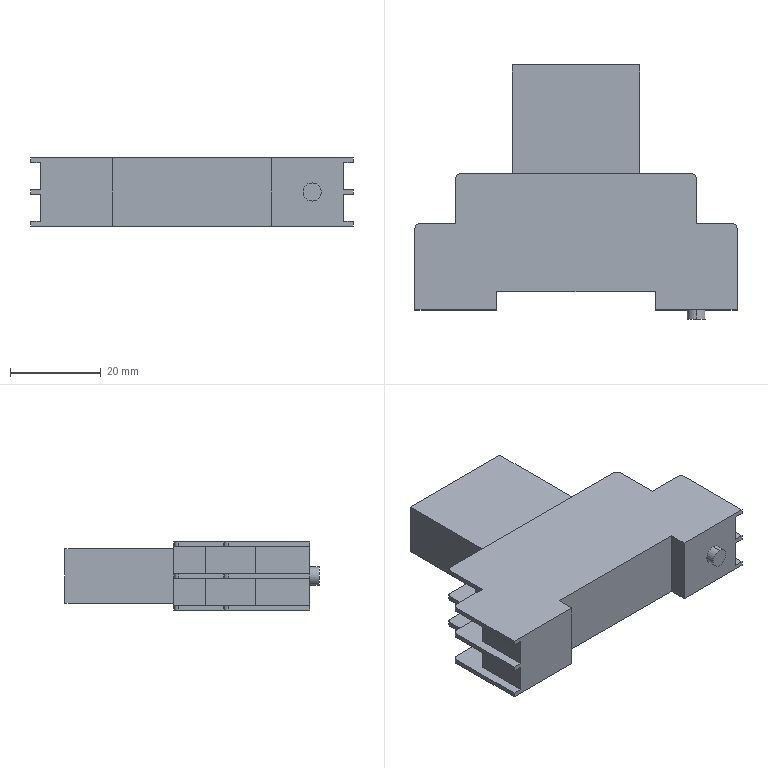Part | STEP file | IDEC relay RJ1S-A220 | 1 solid | 106 faces | box 71 x 56 x 15 mm | volume 30075 mm3 | plane 60 | cylinder 30 | cone 16 | commonest cylinder face diameters 2.5 x16 2 x12 4 x2